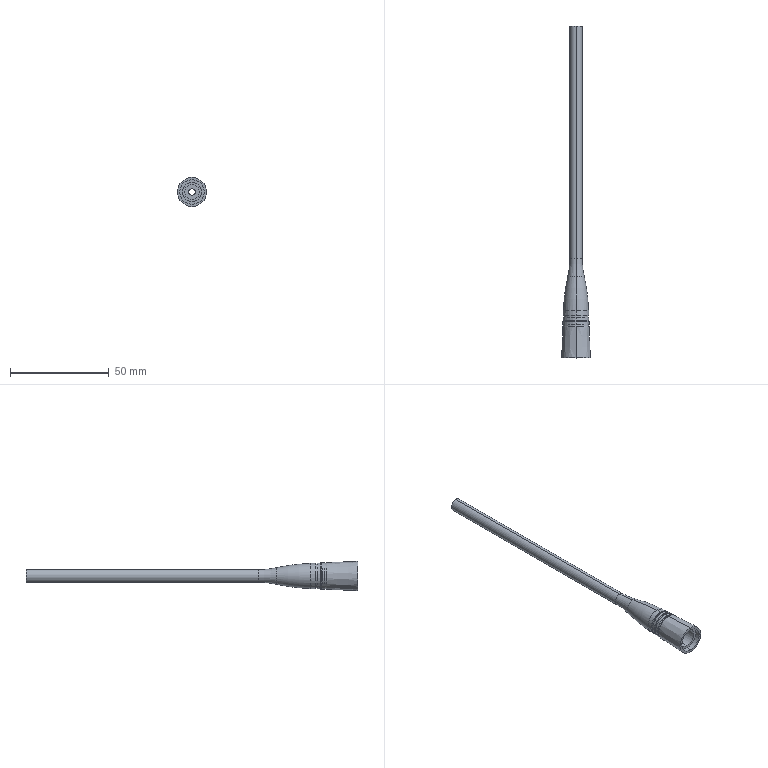Part | SolidWorks | features Fillet 1, Revolution 1 | 1 solid | 69 faces | box 14.8 x 168 x 14.8 mm | volume 6070 mm3 | torus 34 | cone 14 | plane 11 | cylinder 10 | commonest cylinder face diameters 3.3 x2 6.35 x2 7.5 x2 9.5 x2 12.4 x2